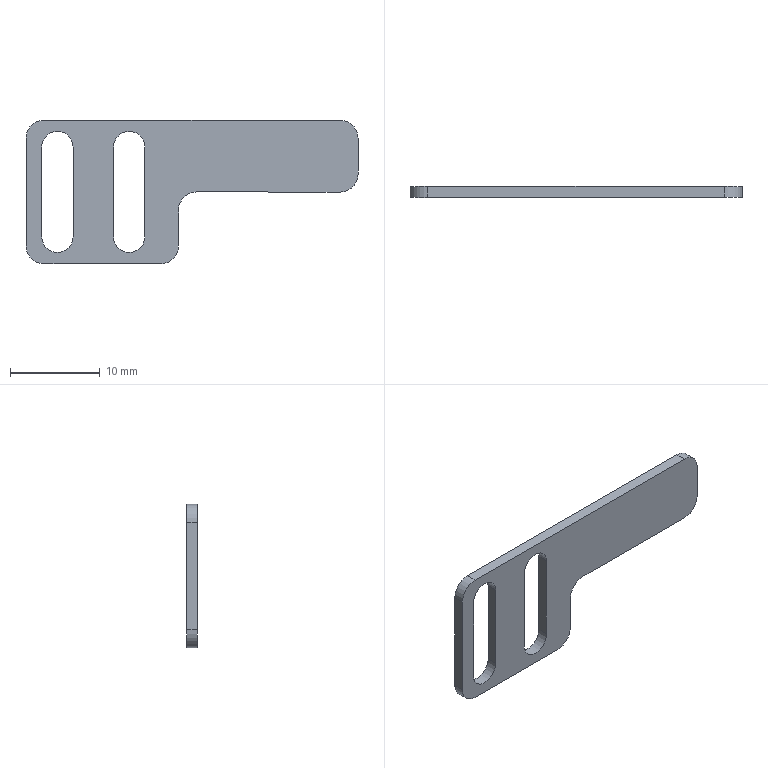Part | SolidWorks | features BaseBody 1 | 1 solid | 24 faces | box 37 x 1.2 x 16 mm | volume 407.189 mm3 | cylinder 12 | plane 12 | commonest cylinder face diameters 3.5 x6 4 x6
STEP:
#1=CARTESIAN_POINT('',(-3.5,-1.2,-8.));
#2=VERTEX_POINT('',#1);
#3=CARTESIAN_POINT('',(-1.5,-1.2,-6.));
#4=VERTEX_POINT('',#3);
#5=CARTESIAN_POINT('',(-3.5,-1.2,-6.));
#6=DIRECTION('',(0.,-1.,0.));
#7=DIRECTION('',(0.,0.,1.));
#8=AXIS2_PLACEMENT_3D('',#5,#6,#7);
#9=CIRCLE('',#8,2.);
#10=EDGE_CURVE('',#2,#4,#9,.T.);
#11=ORIENTED_EDGE('',*,*,#10,.F.);
#12=CARTESIAN_POINT('',(-3.5,0.,-8.));
#13=VERTEX_POINT('',#12);
#14=CARTESIAN_POINT('',(-3.5,-1.2,-8.));
#15=DIRECTION('',(0.,-1.,0.));
#16=VECTOR('',#15,1000.);
#17=LINE('',#14,#16);
#18=EDGE_CURVE('',#13,#2,#17,.T.);
#19=ORIENTED_EDGE('',*,*,#18,.F.);
#20=CARTESIAN_POINT('',(-1.5,0.,-6.));
#21=VERTEX_POINT('',#20);
#22=CARTESIAN_POINT('',(-3.5,0.,-6.));
#23=DIRECTION('',(0.,1.,0.));
#24=DIRECTION('',(0.,0.,1.));
#25=AXIS2_PLACEMENT_3D('',#22,#23,#24);
#26=CIRCLE('',#25,2.);
#27=EDGE_CURVE('',#21,#13,#26,.T.);
#28=ORIENTED_EDGE('',*,*,#27,.F.);
#29=CARTESIAN_POINT('',(-1.5,0.,-6.));
#30=DIRECTION('',(0.,1.,0.));
#31=VECTOR('',#30,1000.);
#32=LINE('',#29,#31);
#33=EDGE_CURVE('',#4,#21,#32,.T.);
#34=ORIENTED_EDGE('',*,*,#33,.F.);
#35=EDGE_LOOP('',(#11,#19,#28,#34));
#36=FACE_OUTER_BOUND('',#35,.T.);
#37=CARTESIAN_POINT('',(-3.5,-1.201,-6.));
#38=DIRECTION('',(0.,-1.,0.));
#39=DIRECTION('',(0.,0.,-1.));
#40=AXIS2_PLACEMENT_3D('',#37,#38,#39);
#41=CYLINDRICAL_SURFACE('',#40,2.);
#42=ADVANCED_FACE('',(#36),#41,.T.);
#43=CARTESIAN_POINT('',(16.5,-1.2,0.));
#44=VERTEX_POINT('',#43);
#45=CARTESIAN_POINT('',(18.5,-1.2,2.));
#46=VERTEX_POINT('',#45);
#47=CARTESIAN_POINT('',(16.5,-1.2,2.));
#48=DIRECTION('',(0.,-1.,0.));
#49=DIRECTION('',(0.,0.,1.));
#50=AXIS2_PLACEMENT_3D('',#47,#48,#49);
#51=CIRCLE('',#50,2.);
#52=EDGE_CURVE('',#44,#46,#51,.T.);
#53=ORIENTED_EDGE('',*,*,#52,.F.);
#54=CARTESIAN_POINT('',(16.5,0.,0.));
#55=VERTEX_POINT('',#54);
#56=CARTESIAN_POINT('',(16.5,-1.2,0.));
#57=DIRECTION('',(0.,-1.,0.));
#58=VECTOR('',#57,1000.);
#59=LINE('',#56,#58);
#60=EDGE_CURVE('',#55,#44,#59,.T.);
#61=ORIENTED_EDGE('',*,*,#60,.F.);
#62=CARTESIAN_POINT('',(18.5,0.,2.));
#63=VERTEX_POINT('',#62);
#64=CARTESIAN_POINT('',(16.5,0.,2.));
#65=DIRECTION('',(0.,1.,0.));
#66=DIRECTION('',(0.,0.,1.));
#67=AXIS2_PLACEMENT_3D('',#64,#65,#66);
#68=CIRCLE('',#67,2.);
#69=EDGE_CURVE('',#63,#55,#68,.T.);
#70=ORIENTED_EDGE('',*,*,#69,.F.);
#71=CARTESIAN_POINT('',(18.5,0.,2.));
#72=DIRECTION('',(0.,1.,0.));
#73=VECTOR('',#72,1000.);
#74=LINE('',#71,#73);
#75=EDGE_CURVE('',#46,#63,#74,.T.);
#76=ORIENTED_EDGE('',*,*,#75,.F.);
#77=EDGE_LOOP('',(#53,#61,#70,#76));
#78=FACE_OUTER_BOUND('',#77,.T.);
#79=CARTESIAN_POINT('',(16.5,-1.2,2.));
#80=DIRECTION('',(0.,-1.,0.));
#81=DIRECTION('',(0.,0.,-1.));
#82=AXIS2_PLACEMENT_3D('',#79,#80,#81);
#83=CYLINDRICAL_SURFACE('',#82,2.);
#84=ADVANCED_FACE('',(#78),#83,.T.);
#85=CARTESIAN_POINT('',(-1.5,-1.2,-2.));
#86=VERTEX_POINT('',#85);
#87=CARTESIAN_POINT('',(0.5,-1.2,0.));
#88=VERTEX_POINT('',#87);
#89=CARTESIAN_POINT('',(0.5,-1.2,-2.));
#90=DIRECTION('',(0.,1.,0.));
#91=DIRECTION('',(0.,0.,1.));
#92=AXIS2_PLACEMENT_3D('',#89,#90,#91);
#93=CIRCLE('',#92,2.);
#94=EDGE_CURVE('',#86,#88,#93,.T.);
#95=ORIENTED_EDGE('',*,*,#94,.F.);
#96=CARTESIAN_POINT('',(-1.5,0.,-2.));
#97=VERTEX_POINT('',#96);
#98=CARTESIAN_POINT('',(-1.5,-1.2,-2.));
#99=DIRECTION('',(0.,-1.,0.));
#100=VECTOR('',#99,1000.);
#101=LINE('',#98,#100);
#102=EDGE_CURVE('',#97,#86,#101,.T.);
#103=ORIENTED_EDGE('',*,*,#102,.F.);
#104=CARTESIAN_POINT('',(0.5,0.,0.));
#105=VERTEX_POINT('',#104);
#106=CARTESIAN_POINT('',(0.5,0.,-2.));
#107=DIRECTION('',(0.,-1.,0.));
#108=DIRECTION('',(0.,0.,1.));
#109=AXIS2_PLACEMENT_3D('',#106,#107,#108);
#110=CIRCLE('',#109,2.);
#111=EDGE_CURVE('',#105,#97,#110,.T.);
#112=ORIENTED_EDGE('',*,*,#111,.F.);
#113=CARTESIAN_POINT('',(0.5,0.,0.));
#114=DIRECTION('',(0.,1.,0.));
#115=VECTOR('',#114,1000.);
#116=LINE('',#113,#115);
#117=EDGE_CURVE('',#88,#105,#116,.T.);
#118=ORIENTED_EDGE('',*,*,#117,.F.);
#119=EDGE_LOOP('',(#95,#103,#112,#118));
#120=FACE_OUTER_BOUND('',#119,.T.);
#121=CARTESIAN_POINT('',(0.5,-1.201,-2.));
#122=DIRECTION('',(0.,-1.,0.));
#123=DIRECTION('',(0.,0.,-1.));
#124=AXIS2_PLACEMENT_3D('',#121,#122,#123);
#125=CYLINDRICAL_SURFACE('',#124,2.);
#126=ADVANCED_FACE('',(#120),#125,.F.);
#127=CARTESIAN_POINT('',(-18.5,-1.2,-6.));
#128=VERTEX_POINT('',#127);
#129=CARTESIAN_POINT('',(-16.5,-1.2,-8.));
#130=VERTEX_POINT('',#129);
#131=CARTESIAN_POINT('',(-16.5,-1.2,-6.));
#132=DIRECTION('',(0.,-1.,0.));
#133=DIRECTION('',(0.,0.,1.));
#134=AXIS2_PLACEMENT_3D('',#131,#132,#133);
#135=CIRCLE('',#134,2.);
#136=EDGE_CURVE('',#128,#130,#135,.T.);
#137=ORIENTED_EDGE('',*,*,#136,.F.);
#138=CARTESIAN_POINT('',(-18.5,0.,-6.));
#139=VERTEX_POINT('',#138);
#140=CARTESIAN_POINT('',(-18.5,-1.2,-6.));
#141=DIRECTION('',(0.,-1.,0.));
#142=VECTOR('',#141,1000.);
#143=LINE('',#140,#142);
#144=EDGE_CURVE('',#139,#128,#143,.T.);
#145=ORIENTED_EDGE('',*,*,#144,.F.);
#146=CARTESIAN_POINT('',(-16.5,0.,-8.));
#147=VERTEX_POINT('',#146);
#148=CARTESIAN_POINT('',(-16.5,0.,-6.));
#149=DIRECTION('',(0.,1.,0.));
#150=DIRECTION('',(0.,0.,1.));
#151=AXIS2_PLACEMENT_3D('',#148,#149,#150);
#152=CIRCLE('',#151,2.);
#153=EDGE_CURVE('',#147,#139,#152,.T.);
#154=ORIENTED_EDGE('',*,*,#153,.F.);
#155=CARTESIAN_POINT('',(-16.5,-1.2,-8.));
#156=DIRECTION('',(0.,1.,0.));
#157=VECTOR('',#156,1000.);
#158=LINE('',#155,#157);
#159=EDGE_CURVE('',#130,#147,#158,.T.);
#160=ORIENTED_EDGE('',*,*,#159,.F.);
#161=EDGE_LOOP('',(#137,#145,#154,#160));
#162=FACE_OUTER_BOUND('',#161,.T.);
#163=CARTESIAN_POINT('',(-16.5,-1.2,-6.));
#164=DIRECTION('',(0.,1.,0.));
#165=DIRECTION('',(0.,0.,1.));
#166=AXIS2_PLACEMENT_3D('',#163,#164,#165);
#167=CYLINDRICAL_SURFACE('',#166,2.);
#168=ADVANCED_FACE('',(#162),#167,.T.);
#169=CARTESIAN_POINT('',(-16.5,-1.2,8.));
#170=VERTEX_POINT('',#169);
#171=CARTESIAN_POINT('',(-18.5,-1.2,6.));
#172=VERTEX_POINT('',#171);
#173=CARTESIAN_POINT('',(-16.5,-1.2,6.));
#174=DIRECTION('',(0.,-1.,0.));
#175=DIRECTION('',(0.,0.,1.));
#176=AXIS2_PLACEMENT_3D('',#173,#174,#175);
#177=CIRCLE('',#176,2.);
#178=EDGE_CURVE('',#170,#172,#177,.T.);
#179=ORIENTED_EDGE('',*,*,#178,.F.);
#180=CARTESIAN_POINT('',(-16.5,0.,8.));
#181=VERTEX_POINT('',#180);
#182=CARTESIAN_POINT('',(-16.5,-1.2,8.));
#183=DIRECTION('',(0.,-1.,0.));
#184=VECTOR('',#183,1000.);
#185=LINE('',#182,#184);
#186=EDGE_CURVE('',#181,#170,#185,.T.);
#187=ORIENTED_EDGE('',*,*,#186,.F.);
#188=CARTESIAN_POINT('',(-18.5,0.,6.));
#189=VERTEX_POINT('',#188);
#190=CARTESIAN_POINT('',(-16.5,0.,6.));
#191=DIRECTION('',(0.,1.,0.));
#192=DIRECTION('',(0.,0.,1.));
#193=AXIS2_PLACEMENT_3D('',#190,#191,#192);
#194=CIRCLE('',#193,2.);
#195=EDGE_CURVE('',#189,#181,#194,.T.);
#196=ORIENTED_EDGE('',*,*,#195,.F.);
#197=CARTESIAN_POINT('',(-18.5,-1.2,6.));
#198=DIRECTION('',(0.,1.,0.));
#199=VECTOR('',#198,1000.);
#200=LINE('',#197,#199);
#201=EDGE_CURVE('',#172,#189,#200,.T.);
#202=ORIENTED_EDGE('',*,*,#201,.F.);
#203=EDGE_LOOP('',(#179,#187,#196,#202));
#204=FACE_OUTER_BOUND('',#203,.T.);
#205=CARTESIAN_POINT('',(-16.5,-1.2,6.));
#206=DIRECTION('',(0.,1.,0.));
#207=DIRECTION('',(0.,0.,1.));
#208=AXIS2_PLACEMENT_3D('',#205,#206,#207);
#209=CYLINDRICAL_SURFACE('',#208,2.);
#210=ADVANCED_FACE('',(#204),#209,.T.);
#211=CARTESIAN_POINT('',(18.5,-1.2,6.));
#212=VERTEX_POINT('',#211);
#213=CARTESIAN_POINT('',(16.5,-1.2,8.));
#214=VERTEX_POINT('',#213);
#215=CARTESIAN_POINT('',(16.5,-1.2,6.));
#216=DIRECTION('',(0.,-1.,0.));
#217=DIRECTION('',(0.,0.,1.));
#218=AXIS2_PLACEMENT_3D('',#215,#216,#217);
#219=CIRCLE('',#218,2.);
#220=EDGE_CURVE('',#212,#214,#219,.T.);
#221=ORIENTED_EDGE('',*,*,#220,.F.);
#222=CARTESIAN_POINT('',(18.5,0.,6.));
#223=VERTEX_POINT('',#222);
#224=CARTESIAN_POINT('',(18.5,-1.2,6.));
#225=DIRECTION('',(0.,-1.,0.));
#226=VECTOR('',#225,1000.);
#227=LINE('',#224,#226);
#228=EDGE_CURVE('',#223,#212,#227,.T.);
#229=ORIENTED_EDGE('',*,*,#228,.F.);
#230=CARTESIAN_POINT('',(16.5,0.,8.));
#231=VERTEX_POINT('',#230);
#232=CARTESIAN_POINT('',(16.5,0.,6.));
#233=DIRECTION('',(0.,1.,0.));
#234=DIRECTION('',(0.,0.,1.));
#235=AXIS2_PLACEMENT_3D('',#232,#233,#234);
#236=CIRCLE('',#235,2.);
#237=EDGE_CURVE('',#231,#223,#236,.T.);
#238=ORIENTED_EDGE('',*,*,#237,.F.);
#239=CARTESIAN_POINT('',(16.5,-1.2,8.));
#240=DIRECTION('',(0.,1.,0.));
#241=VECTOR('',#240,1000.);
#242=LINE('',#239,#241);
#243=EDGE_CURVE('',#214,#231,#242,.T.);
#244=ORIENTED_EDGE('',*,*,#243,.F.);
#245=EDGE_LOOP('',(#221,#229,#238,#244));
#246=FACE_OUTER_BOUND('',#245,.T.);
#247=CARTESIAN_POINT('',(16.5,-1.2,6.));
#248=DIRECTION('',(0.,1.,0.));
#249=DIRECTION('',(0.,0.,1.));
#250=AXIS2_PLACEMENT_3D('',#247,#248,#249);
#251=CYLINDRICAL_SURFACE('',#250,2.);
#252=ADVANCED_FACE('',(#246),#251,.T.);
#253=CARTESIAN_POINT('',(-1.5,0.,-8.));
#254=DIRECTION('',(0.,0.,1.));
#255=VECTOR('',#254,1000.);
#256=LINE('',#253,#255);
#257=EDGE_CURVE('',#21,#97,#256,.T.);
#258=ORIENTED_EDGE('',*,*,#257,.T.);
#259=ORIENTED_EDGE('',*,*,#102,.T.);
#260=CARTESIAN_POINT('',(-1.5,-1.2,-8.));
#261=DIRECTION('',(0.,0.,-1.));
#262=VECTOR('',#261,1000.);
#263=LINE('',#260,#262);
#264=EDGE_CURVE('',#86,#4,#263,.T.);
#265=ORIENTED_EDGE('',*,*,#264,.T.);
#266=ORIENTED_EDGE('',*,*,#33,.T.);
#267=EDGE_LOOP('',(#258,#259,#265,#266));
#268=FACE_OUTER_BOUND('',#267,.T.);
#269=CARTESIAN_POINT('',(-1.5,-1.201,-8.));
#270=DIRECTION('',(-1.,0.,0.));
#271=DIRECTION('',(0.,1.,0.));
#272=AXIS2_PLACEMENT_3D('',#269,#270,#271);
#273=PLANE('',#272);
#274=ADVANCED_FACE('',(#268),#273,.F.);
#275=CARTESIAN_POINT('',(18.5,-1.2,0.));
#276=DIRECTION('',(-1.,0.,0.));
#277=VECTOR('',#276,1000.);
#278=LINE('',#275,#277);
#279=EDGE_CURVE('',#44,#88,#278,.T.);
#280=ORIENTED_EDGE('',*,*,#279,.T.);
#281=ORIENTED_EDGE('',*,*,#117,.T.);
#282=CARTESIAN_POINT('',(18.5,0.,0.));
#283=DIRECTION('',(1.,0.,0.));
#284=VECTOR('',#283,1000.);
#285=LINE('',#282,#284);
#286=EDGE_CURVE('',#105,#55,#285,.T.);
#287=ORIENTED_EDGE('',*,*,#286,.T.);
#288=ORIENTED_EDGE('',*,*,#60,.T.);
#289=EDGE_LOOP('',(#280,#281,#287,#288));
#290=FACE_OUTER_BOUND('',#289,.T.);
#291=CARTESIAN_POINT('',(18.5,-1.201,0.));
#292=DIRECTION('',(0.,0.,1.));
#293=DIRECTION('',(1.,0.,0.));
#294=AXIS2_PLACEMENT_3D('',#291,#292,#293);
#295=PLANE('',#294);
#296=ADVANCED_FACE('',(#290),#295,.F.);
#297=CARTESIAN_POINT('',(-16.75,-1.2,5.));
#298=VERTEX_POINT('',#297);
#299=CARTESIAN_POINT('',(-16.75,-1.2,-5.));
#300=VERTEX_POINT('',#299);
#301=CARTESIAN_POINT('',(-16.75,-1.2,-5.));
#302=DIRECTION('',(0.,0.,-1.));
#303=VECTOR('',#302,1000.);
#304=LINE('',#301,#303);
#305=EDGE_CURVE('',#298,#300,#304,.T.);
#306=ORIENTED_EDGE('',*,*,#305,.T.);
#307=CARTESIAN_POINT('',(-16.75,0.,-5.));
#308=VERTEX_POINT('',#307);
#309=CARTESIAN_POINT('',(-16.75,-1.201,-5.));
#310=DIRECTION('',(0.,1.,0.));
#311=VECTOR('',#310,1000.);
#312=LINE('',#309,#311);
#313=EDGE_CURVE('',#300,#308,#312,.T.);
#314=ORIENTED_EDGE('',*,*,#313,.T.);
#315=CARTESIAN_POINT('',(-16.75,0.,5.));
#316=VERTEX_POINT('',#315);
#317=CARTESIAN_POINT('',(-16.75,0.,-5.));
#318=DIRECTION('',(0.,0.,1.));
#319=VECTOR('',#318,1000.);
#320=LINE('',#317,#319);
#321=EDGE_CURVE('',#308,#316,#320,.T.);
#322=ORIENTED_EDGE('',*,*,#321,.T.);
#323=CARTESIAN_POINT('',(-16.75,-1.201,5.));
#324=DIRECTION('',(0.,1.,0.));
#325=VECTOR('',#324,1000.);
#326=LINE('',#323,#325);
#327=EDGE_CURVE('',#298,#316,#326,.T.);
#328=ORIENTED_EDGE('',*,*,#327,.F.);
#329=EDGE_LOOP('',(#306,#314,#322,#328));
#330=FACE_OUTER_BOUND('',#329,.T.);
#331=CARTESIAN_POINT('',(-16.75,-1.201,-5.));
#332=DIRECTION('',(-1.,0.,0.));
#333=DIRECTION('',(0.,0.,1.));
#334=AXIS2_PLACEMENT_3D('',#331,#332,#333);
#335=PLANE('',#334);
#336=ADVANCED_FACE('',(#330),#335,.F.);
#337=CARTESIAN_POINT('',(-15.,-1.2,6.75));
#338=VERTEX_POINT('',#337);
#339=CARTESIAN_POINT('',(-15.,0.,6.75));
#340=VERTEX_POINT('',#339);
#341=CARTESIAN_POINT('',(-15.,-1.201,6.75));
#342=DIRECTION('',(0.,1.,0.));
#343=VECTOR('',#342,1000.);
#344=LINE('',#341,#343);
#345=EDGE_CURVE('',#338,#340,#344,.T.);
#346=ORIENTED_EDGE('',*,*,#345,.F.);
#347=CARTESIAN_POINT('',(-15.,-1.2,5.));
#348=DIRECTION('',(0.,-1.,0.));
#349=DIRECTION('',(0.,0.,1.));
#350=AXIS2_PLACEMENT_3D('',#347,#348,#349);
#351=CIRCLE('',#350,1.75);
#352=EDGE_CURVE('',#338,#298,#351,.T.);
#353=ORIENTED_EDGE('',*,*,#352,.T.);
#354=ORIENTED_EDGE('',*,*,#327,.T.);
#355=CARTESIAN_POINT('',(-15.,0.,5.));
#356=DIRECTION('',(0.,1.,0.));
#357=DIRECTION('',(0.,0.,1.));
#358=AXIS2_PLACEMENT_3D('',#355,#356,#357);
#359=CIRCLE('',#358,1.75);
#360=EDGE_CURVE('',#316,#340,#359,.T.);
#361=ORIENTED_EDGE('',*,*,#360,.T.);
#362=EDGE_LOOP('',(#346,#353,#354,#361));
#363=FACE_OUTER_BOUND('',#362,.T.);
#364=CARTESIAN_POINT('',(-15.,-1.201,5.));
#365=DIRECTION('',(0.,1.,0.));
#366=DIRECTION('',(0.,0.,1.));
#367=AXIS2_PLACEMENT_3D('',#364,#365,#366);
#368=CYLINDRICAL_SURFACE('',#367,1.75);
#369=ADVANCED_FACE('',(#363),#368,.F.);
#370=CARTESIAN_POINT('',(-13.25,-1.2,-5.));
#371=VERTEX_POINT('',#370);
#372=CARTESIAN_POINT('',(-13.25,-1.2,5.));
#373=VERTEX_POINT('',#372);
#374=CARTESIAN_POINT('',(-13.25,-1.2,-5.));
#375=DIRECTION('',(0.,0.,1.));
#376=VECTOR('',#375,1000.);
#377=LINE('',#374,#376);
#378=EDGE_CURVE('',#371,#373,#377,.T.);
#379=ORIENTED_EDGE('',*,*,#378,.T.);
#380=CARTESIAN_POINT('',(-13.25,0.,5.));
#381=VERTEX_POINT('',#380);
#382=CARTESIAN_POINT('',(-13.25,-1.201,5.));
#383=DIRECTION('',(0.,1.,0.));
#384=VECTOR('',#383,1000.);
#385=LINE('',#382,#384);
#386=EDGE_CURVE('',#373,#381,#385,.T.);
#387=ORIENTED_EDGE('',*,*,#386,.T.);
#388=CARTESIAN_POINT('',(-13.25,0.,-5.));
#389=VERTEX_POINT('',#388);
#390=CARTESIAN_POINT('',(-13.25,0.,-5.));
#391=DIRECTION('',(0.,0.,-1.));
#392=VECTOR('',#391,1000.);
#393=LINE('',#390,#392);
#394=EDGE_CURVE('',#381,#389,#393,.T.);
#395=ORIENTED_EDGE('',*,*,#394,.T.);
#396=CARTESIAN_POINT('',(-13.25,-1.201,-5.));
#397=DIRECTION('',(0.,1.,0.));
#398=VECTOR('',#397,1000.);
#399=LINE('',#396,#398);
#400=EDGE_CURVE('',#371,#389,#399,.T.);
#401=ORIENTED_EDGE('',*,*,#400,.F.);
#402=EDGE_LOOP('',(#379,#387,#395,#401));
#403=FACE_OUTER_BOUND('',#402,.T.);
#404=CARTESIAN_POINT('',(-13.25,-1.201,-5.));
#405=DIRECTION('',(1.,0.,0.));
#406=DIRECTION('',(0.,1.,0.));
#407=AXIS2_PLACEMENT_3D('',#404,#405,#406);
#408=PLANE('',#407);
#409=ADVANCED_FACE('',(#403),#408,.F.);
#410=CARTESIAN_POINT('',(-15.,-1.2,-5.));
#411=DIRECTION('',(0.,-1.,0.));
#412=DIRECTION('',(0.,0.,1.));
#413=AXIS2_PLACEMENT_3D('',#410,#411,#412);
#414=CIRCLE('',#413,1.75);
#415=EDGE_CURVE('',#300,#371,#414,.T.);
#416=ORIENTED_EDGE('',*,*,#415,.T.);
#417=ORIENTED_EDGE('',*,*,#400,.T.);
#418=CARTESIAN_POINT('',(-15.,0.,-5.));
#419=DIRECTION('',(0.,1.,0.));
#420=DIRECTION('',(0.,0.,1.));
#421=AXIS2_PLACEMENT_3D('',#418,#419,#420);
#422=CIRCLE('',#421,1.75);
#423=EDGE_CURVE('',#389,#308,#422,.T.);
#424=ORIENTED_EDGE('',*,*,#423,.T.);
#425=ORIENTED_EDGE('',*,*,#313,.F.);
#426=EDGE_LOOP('',(#416,#417,#424,#425));
#427=FACE_OUTER_BOUND('',#426,.T.);
#428=CARTESIAN_POINT('',(-15.,-1.201,-5.));
#429=DIRECTION('',(0.,1.,0.));
#430=DIRECTION('',(0.,0.,1.));
#431=AXIS2_PLACEMENT_3D('',#428,#429,#430);
#432=CYLINDRICAL_SURFACE('',#431,1.75);
#433=ADVANCED_FACE('',(#427),#432,.F.);
#434=CARTESIAN_POINT('',(-8.75,-1.2,5.));
#435=VERTEX_POINT('',#434);
#436=CARTESIAN_POINT('',(-8.75,-1.2,-5.));
#437=VERTEX_POINT('',#436);
#438=CARTESIAN_POINT('',(-8.75,-1.2,-5.));
#439=DIRECTION('',(0.,0.,-1.));
#440=VECTOR('',#439,1000.);
#441=LINE('',#438,#440);
#442=EDGE_CURVE('',#435,#437,#441,.T.);
#443=ORIENTED_EDGE('',*,*,#442,.T.);
#444=CARTESIAN_POINT('',(-8.75,0.,-5.));
#445=VERTEX_POINT('',#444);
#446=CARTESIAN_POINT('',(-8.75,-1.201,-5.));
#447=DIRECTION('',(0.,1.,0.));
#448=VECTOR('',#447,1000.);
#449=LINE('',#446,#448);
#450=EDGE_CURVE('',#437,#445,#449,.T.);
#451=ORIENTED_EDGE('',*,*,#450,.T.);
#452=CARTESIAN_POINT('',(-8.75,0.,5.));
#453=VERTEX_POINT('',#452);
#454=CARTESIAN_POINT('',(-8.75,0.,-5.));
#455=DIRECTION('',(0.,0.,1.));
#456=VECTOR('',#455,1000.);
#457=LINE('',#454,#456);
#458=EDGE_CURVE('',#445,#453,#457,.T.);
#459=ORIENTED_EDGE('',*,*,#458,.T.);
#460=CARTESIAN_POINT('',(-8.75,-1.201,5.));
#461=DIRECTION('',(0.,1.,0.));
#462=VECTOR('',#461,1000.);
#463=LINE('',#460,#462);
#464=EDGE_CURVE('',#435,#453,#463,.T.);
#465=ORIENTED_EDGE('',*,*,#464,.F.);
#466=EDGE_LOOP('',(#443,#451,#459,#465));
#467=FACE_OUTER_BOUND('',#466,.T.);
#468=CARTESIAN_POINT('',(-8.75,-1.201,-5.));
#469=DIRECTION('',(-1.,0.,0.));
#470=DIRECTION('',(0.,0.,1.));
#471=AXIS2_PLACEMENT_3D('',#468,#469,#470);
#472=PLANE('',#471);
#473=ADVANCED_FACE('',(#467),#472,.F.);
#474=CARTESIAN_POINT('',(-7.,-1.2,6.75));
#475=VERTEX_POINT('',#474);
#476=CARTESIAN_POINT('',(-7.,0.,6.75));
#477=VERTEX_POINT('',#476);
#478=CARTESIAN_POINT('',(-7.,-1.201,6.75));
#479=DIRECTION('',(0.,1.,0.));
#480=VECTOR('',#479,1000.);
#481=LINE('',#478,#480);
#482=EDGE_CURVE('',#475,#477,#481,.T.);
#483=ORIENTED_EDGE('',*,*,#482,.F.);
#484=CARTESIAN_POINT('',(-7.,-1.2,5.));
#485=DIRECTION('',(0.,-1.,0.));
#486=DIRECTION('',(0.,0.,1.));
#487=AXIS2_PLACEMENT_3D('',#484,#485,#486);
#488=CIRCLE('',#487,1.75);
#489=EDGE_CURVE('',#475,#435,#488,.T.);
#490=ORIENTED_EDGE('',*,*,#489,.T.);
#491=ORIENTED_EDGE('',*,*,#464,.T.);
#492=CARTESIAN_POINT('',(-7.,0.,5.));
#493=DIRECTION('',(0.,1.,0.));
#494=DIRECTION('',(0.,0.,1.));
#495=AXIS2_PLACEMENT_3D('',#492,#493,#494);
#496=CIRCLE('',#495,1.75);
#497=EDGE_CURVE('',#453,#477,#496,.T.);
#498=ORIENTED_EDGE('',*,*,#497,.T.);
#499=EDGE_LOOP('',(#483,#490,#491,#498));
#500=FACE_OUTER_BOUND('',#499,.T.);
#501=CARTESIAN_POINT('',(-7.,-1.201,5.));
#502=DIRECTION('',(0.,1.,0.));
#503=DIRECTION('',(0.,0.,1.));
#504=AXIS2_PLACEMENT_3D('',#501,#502,#503);
#505=CYLINDRICAL_SURFACE('',#504,1.75);
#506=ADVANCED_FACE('',(#500),#505,.F.);
#507=CARTESIAN_POINT('',(-5.25,-1.2,-5.));
#508=VERTEX_POINT('',#507);
#509=CARTESIAN_POINT('',(-5.25,-1.2,5.));
#510=VERTEX_POINT('',#509);
#511=CARTESIAN_POINT('',(-5.25,-1.2,-5.));
#512=DIRECTION('',(0.,0.,1.));
#513=VECTOR('',#512,1000.);
#514=LINE('',#511,#513);
#515=EDGE_CURVE('',#508,#510,#514,.T.);
#516=ORIENTED_EDGE('',*,*,#515,.T.);
#517=CARTESIAN_POINT('',(-5.25,0.,5.));
#518=VERTEX_POINT('',#517);
#519=CARTESIAN_POINT('',(-5.25,-1.201,5.));
#520=DIRECTION('',(0.,1.,0.));
#521=VECTOR('',#520,1000.);
#522=LINE('',#519,#521);
#523=EDGE_CURVE('',#510,#518,#522,.T.);
#524=ORIENTED_EDGE('',*,*,#523,.T.);
#525=CARTESIAN_POINT('',(-5.25,0.,-5.));
#526=VERTEX_POINT('',#525);
#527=CARTESIAN_POINT('',(-5.25,0.,-5.));
#528=DIRECTION('',(0.,0.,-1.));
#529=VECTOR('',#528,1000.);
#530=LINE('',#527,#529);
#531=EDGE_CURVE('',#518,#526,#530,.T.);
#532=ORIENTED_EDGE('',*,*,#531,.T.);
#533=CARTESIAN_POINT('',(-5.25,-1.201,-5.));
#534=DIRECTION('',(0.,1.,0.));
#535=VECTOR('',#534,1000.);
#536=LINE('',#533,#535);
#537=EDGE_CURVE('',#508,#526,#536,.T.);
#538=ORIENTED_EDGE('',*,*,#537,.F.);
#539=EDGE_LOOP('',(#516,#524,#532,#538));
#540=FACE_OUTER_BOUND('',#539,.T.);
#541=CARTESIAN_POINT('',(-5.25,-1.201,-5.));
#542=DIRECTION('',(1.,0.,0.));
#543=DIRECTION('',(0.,1.,0.));
#544=AXIS2_PLACEMENT_3D('',#541,#542,#543);
#545=PLANE('',#544);
#546=ADVANCED_FACE('',(#540),#545,.F.);
#547=CARTESIAN_POINT('',(-7.,-1.2,-5.));
#548=DIRECTION('',(0.,-1.,0.));
#549=DIRECTION('',(0.,0.,1.));
#550=AXIS2_PLACEMENT_3D('',#547,#548,#549);
#551=CIRCLE('',#550,1.75);
#552=EDGE_CURVE('',#437,#508,#551,.T.);
#553=ORIENTED_EDGE('',*,*,#552,.T.);
#554=ORIENTED_EDGE('',*,*,#537,.T.);
#555=CARTESIAN_POINT('',(-7.,0.,-5.));
#556=DIRECTION('',(0.,1.,0.));
#557=DIRECTION('',(0.,0.,1.));
#558=AXIS2_PLACEMENT_3D('',#555,#556,#557);
#559=CIRCLE('',#558,1.75);
#560=EDGE_CURVE('',#526,#445,#559,.T.);
#561=ORIENTED_EDGE('',*,*,#560,.T.);
#562=ORIENTED_EDGE('',*,*,#450,.F.);
#563=EDGE_LOOP('',(#553,#554,#561,#562));
#564=FACE_OUTER_BOUND('',#563,.T.);
#565=CARTESIAN_POINT('',(-7.,-1.201,-5.));
#566=DIRECTION('',(0.,1.,0.));
#567=DIRECTION('',(0.,0.,1.));
#568=AXIS2_PLACEMENT_3D('',#565,#566,#567);
#569=CYLINDRICAL_SURFACE('',#568,1.75);
#570=ADVANCED_FACE('',(#564),#569,.F.);
#571=ORIENTED_EDGE('',*,*,#560,.F.);
#572=ORIENTED_EDGE('',*,*,#531,.F.);
#573=CARTESIAN_POINT('',(-7.,0.,5.));
#574=DIRECTION('',(0.,1.,0.));
#575=DIRECTION('',(0.,0.,1.));
#576=AXIS2_PLACEMENT_3D('',#573,#574,#575);
#577=CIRCLE('',#576,1.75);
#578=EDGE_CURVE('',#477,#518,#577,.T.);
#579=ORIENTED_EDGE('',*,*,#578,.F.);
#580=ORIENTED_EDGE('',*,*,#497,.F.);
#581=ORIENTED_EDGE('',*,*,#458,.F.);
#582=EDGE_LOOP('',(#571,#572,#579,#580,#581));
#583=FACE_BOUND('',#582,.T.);
#584=ORIENTED_EDGE('',*,*,#423,.F.);
#585=ORIENTED_EDGE('',*,*,#394,.F.);
#586=CARTESIAN_POINT('',(-15.,0.,5.));
#587=DIRECTION('',(0.,1.,0.));
#588=DIRECTION('',(0.,0.,1.));
#589=AXIS2_PLACEMENT_3D('',#586,#587,#588);
#590=CIRCLE('',#589,1.75);
#591=EDGE_CURVE('',#340,#381,#590,.T.);
#592=ORIENTED_EDGE('',*,*,#591,.F.);
#593=ORIENTED_EDGE('',*,*,#360,.F.);
#594=ORIENTED_EDGE('',*,*,#321,.F.);
#595=EDGE_LOOP('',(#584,#585,#592,#593,#594));
#596=FACE_BOUND('',#595,.T.);
#597=CARTESIAN_POINT('',(-18.5,0.,8.));
#598=DIRECTION('',(1.,0.,0.));
#599=VECTOR('',#598,1000.);
#600=LINE('',#597,#599);
#601=EDGE_CURVE('',#181,#231,#600,.T.);
#602=ORIENTED_EDGE('',*,*,#601,.T.);
#603=ORIENTED_EDGE('',*,*,#237,.T.);
#604=CARTESIAN_POINT('',(18.5,0.,-8.));
#605=DIRECTION('',(0.,0.,-1.));
#606=VECTOR('',#605,1000.);
#607=LINE('',#604,#606);
#608=EDGE_CURVE('',#223,#63,#607,.T.);
#609=ORIENTED_EDGE('',*,*,#608,.T.);
#610=ORIENTED_EDGE('',*,*,#69,.T.);
#611=ORIENTED_EDGE('',*,*,#286,.F.);
#612=ORIENTED_EDGE('',*,*,#111,.T.);
#613=ORIENTED_EDGE('',*,*,#257,.F.);
#614=ORIENTED_EDGE('',*,*,#27,.T.);
#615=CARTESIAN_POINT('',(-18.5,0.,-8.));
#616=DIRECTION('',(-1.,0.,0.));
#617=VECTOR('',#616,1000.);
#618=LINE('',#615,#617);
#619=EDGE_CURVE('',#13,#147,#618,.T.);
#620=ORIENTED_EDGE('',*,*,#619,.T.);
#621=ORIENTED_EDGE('',*,*,#153,.T.);
#622=CARTESIAN_POINT('',(-18.5,0.,-8.));
#623=DIRECTION('',(0.,0.,1.));
#624=VECTOR('',#623,1000.);
#625=LINE('',#622,#624);
#626=EDGE_CURVE('',#139,#189,#625,.T.);
#627=ORIENTED_EDGE('',*,*,#626,.T.);
#628=ORIENTED_EDGE('',*,*,#195,.T.);
#629=EDGE_LOOP('',(#602,#603,#609,#610,#611,#612,#613,#614,#620,#621,#627,#628));
#630=FACE_OUTER_BOUND('',#629,.T.);
#631=CARTESIAN_POINT('',(0.,0.,0.));
#632=DIRECTION('',(0.,1.,0.));
#633=DIRECTION('',(1.,0.,0.));
#634=AXIS2_PLACEMENT_3D('',#631,#632,#633);
#635=PLANE('',#634);
#636=ADVANCED_FACE('',(#583,#596,#630),#635,.T.);
#637=ORIENTED_EDGE('',*,*,#515,.F.);
#638=ORIENTED_EDGE('',*,*,#552,.F.);
#639=ORIENTED_EDGE('',*,*,#442,.F.);
#640=ORIENTED_EDGE('',*,*,#489,.F.);
#641=CARTESIAN_POINT('',(-7.,-1.2,5.));
#642=DIRECTION('',(0.,-1.,0.));
#643=DIRECTION('',(0.,0.,1.));
#644=AXIS2_PLACEMENT_3D('',#641,#642,#643);
#645=CIRCLE('',#644,1.75);
#646=EDGE_CURVE('',#510,#475,#645,.T.);
#647=ORIENTED_EDGE('',*,*,#646,.F.);
#648=EDGE_LOOP('',(#637,#638,#639,#640,#647));
#649=FACE_BOUND('',#648,.T.);
#650=ORIENTED_EDGE('',*,*,#378,.F.);
#651=ORIENTED_EDGE('',*,*,#415,.F.);
#652=ORIENTED_EDGE('',*,*,#305,.F.);
#653=ORIENTED_EDGE('',*,*,#352,.F.);
#654=CARTESIAN_POINT('',(-15.,-1.2,5.));
#655=DIRECTION('',(0.,-1.,0.));
#656=DIRECTION('',(0.,0.,1.));
#657=AXIS2_PLACEMENT_3D('',#654,#655,#656);
#658=CIRCLE('',#657,1.75);
#659=EDGE_CURVE('',#373,#338,#658,.T.);
#660=ORIENTED_EDGE('',*,*,#659,.F.);
#661=EDGE_LOOP('',(#650,#651,#652,#653,#660));
#662=FACE_BOUND('',#661,.T.);
#663=CARTESIAN_POINT('',(18.5,-1.2,-8.));
#664=DIRECTION('',(0.,0.,-1.));
#665=VECTOR('',#664,1000.);
#666=LINE('',#663,#665);
#667=EDGE_CURVE('',#212,#46,#666,.T.);
#668=ORIENTED_EDGE('',*,*,#667,.F.);
#669=ORIENTED_EDGE('',*,*,#220,.T.);
#670=CARTESIAN_POINT('',(-18.5,-1.2,8.));
#671=DIRECTION('',(1.,0.,0.));
#672=VECTOR('',#671,1000.);
#673=LINE('',#670,#672);
#674=EDGE_CURVE('',#170,#214,#673,.T.);
#675=ORIENTED_EDGE('',*,*,#674,.F.);
#676=ORIENTED_EDGE('',*,*,#178,.T.);
#677=CARTESIAN_POINT('',(-18.5,-1.2,-8.));
#678=DIRECTION('',(0.,0.,1.));
#679=VECTOR('',#678,1000.);
#680=LINE('',#677,#679);
#681=EDGE_CURVE('',#128,#172,#680,.T.);
#682=ORIENTED_EDGE('',*,*,#681,.F.);
#683=ORIENTED_EDGE('',*,*,#136,.T.);
#684=CARTESIAN_POINT('',(-18.5,-1.2,-8.));
#685=DIRECTION('',(-1.,0.,0.));
#686=VECTOR('',#685,1000.);
#687=LINE('',#684,#686);
#688=EDGE_CURVE('',#2,#130,#687,.T.);
#689=ORIENTED_EDGE('',*,*,#688,.F.);
#690=ORIENTED_EDGE('',*,*,#10,.T.);
#691=ORIENTED_EDGE('',*,*,#264,.F.);
#692=ORIENTED_EDGE('',*,*,#94,.T.);
#693=ORIENTED_EDGE('',*,*,#279,.F.);
#694=ORIENTED_EDGE('',*,*,#52,.T.);
#695=EDGE_LOOP('',(#668,#669,#675,#676,#682,#683,#689,#690,#691,#692,#693,#694));
#696=FACE_OUTER_BOUND('',#695,.T.);
#697=CARTESIAN_POINT('',(0.,-1.2,0.));
#698=DIRECTION('',(0.,1.,0.));
#699=DIRECTION('',(1.,0.,0.));
#700=AXIS2_PLACEMENT_3D('',#697,#698,#699);
#701=PLANE('',#700);
#702=ADVANCED_FACE('',(#649,#662,#696),#701,.F.);
#703=ORIENTED_EDGE('',*,*,#688,.T.);
#704=ORIENTED_EDGE('',*,*,#159,.T.);
#705=ORIENTED_EDGE('',*,*,#619,.F.);
#706=ORIENTED_EDGE('',*,*,#18,.T.);
#707=EDGE_LOOP('',(#703,#704,#705,#706));
#708=FACE_OUTER_BOUND('',#707,.T.);
#709=CARTESIAN_POINT('',(-18.5,-1.2,-8.));
#710=DIRECTION('',(0.,0.,-1.));
#711=DIRECTION('',(0.,-1.,0.));
#712=AXIS2_PLACEMENT_3D('',#709,#710,#711);
#713=PLANE('',#712);
#714=ADVANCED_FACE('',(#708),#713,.T.);
#715=ORIENTED_EDGE('',*,*,#681,.T.);
#716=ORIENTED_EDGE('',*,*,#201,.T.);
#717=ORIENTED_EDGE('',*,*,#626,.F.);
#718=ORIENTED_EDGE('',*,*,#144,.T.);
#719=EDGE_LOOP('',(#715,#716,#717,#718));
#720=FACE_OUTER_BOUND('',#719,.T.);
#721=CARTESIAN_POINT('',(-18.5,-1.2,-8.));
#722=DIRECTION('',(-1.,0.,0.));
#723=DIRECTION('',(0.,1.,0.));
#724=AXIS2_PLACEMENT_3D('',#721,#722,#723);
#725=PLANE('',#724);
#726=ADVANCED_FACE('',(#720),#725,.T.);
#727=ORIENTED_EDGE('',*,*,#674,.T.);
#728=ORIENTED_EDGE('',*,*,#243,.T.);
#729=ORIENTED_EDGE('',*,*,#601,.F.);
#730=ORIENTED_EDGE('',*,*,#186,.T.);
#731=EDGE_LOOP('',(#727,#728,#729,#730));
#732=FACE_OUTER_BOUND('',#731,.T.);
#733=CARTESIAN_POINT('',(-18.5,-1.2,8.));
#734=DIRECTION('',(0.,0.,1.));
#735=DIRECTION('',(1.,0.,0.));
#736=AXIS2_PLACEMENT_3D('',#733,#734,#735);
#737=PLANE('',#736);
#738=ADVANCED_FACE('',(#732),#737,.T.);
#739=ORIENTED_EDGE('',*,*,#608,.F.);
#740=ORIENTED_EDGE('',*,*,#228,.T.);
#741=ORIENTED_EDGE('',*,*,#667,.T.);
#742=ORIENTED_EDGE('',*,*,#75,.T.);
#743=EDGE_LOOP('',(#739,#740,#741,#742));
#744=FACE_OUTER_BOUND('',#743,.T.);
#745=CARTESIAN_POINT('',(18.5,-1.2,-8.));
#746=DIRECTION('',(1.,0.,0.));
#747=DIRECTION('',(0.,0.,1.));
#748=AXIS2_PLACEMENT_3D('',#745,#746,#747);
#749=PLANE('',#748);
#750=ADVANCED_FACE('',(#744),#749,.T.);
#751=ORIENTED_EDGE('',*,*,#646,.T.);
#752=ORIENTED_EDGE('',*,*,#482,.T.);
#753=ORIENTED_EDGE('',*,*,#578,.T.);
#754=ORIENTED_EDGE('',*,*,#523,.F.);
#755=EDGE_LOOP('',(#751,#752,#753,#754));
#756=FACE_OUTER_BOUND('',#755,.T.);
#757=CARTESIAN_POINT('',(-7.,-1.201,5.));
#758=DIRECTION('',(0.,1.,0.));
#759=DIRECTION('',(0.,0.,1.));
#760=AXIS2_PLACEMENT_3D('',#757,#758,#759);
#761=CYLINDRICAL_SURFACE('',#760,1.75);
#762=ADVANCED_FACE('',(#756),#761,.F.);
#763=ORIENTED_EDGE('',*,*,#659,.T.);
#764=ORIENTED_EDGE('',*,*,#345,.T.);
#765=ORIENTED_EDGE('',*,*,#591,.T.);
#766=ORIENTED_EDGE('',*,*,#386,.F.);
#767=EDGE_LOOP('',(#763,#764,#765,#766));
#768=FACE_OUTER_BOUND('',#767,.T.);
#769=CARTESIAN_POINT('',(-15.,-1.201,5.));
#770=DIRECTION('',(0.,1.,0.));
#771=DIRECTION('',(0.,0.,1.));
#772=AXIS2_PLACEMENT_3D('',#769,#770,#771);
#773=CYLINDRICAL_SURFACE('',#772,1.75);
#774=ADVANCED_FACE('',(#768),#773,.F.);
#775=CLOSED_SHELL('',(#42,#84,#126,#168,#210,#252,#274,#296,#336,#369,#409,#433,#473,#506,#546,#570,#636,#702,#714,#726,#738,#750,#762,#774));
#776=MANIFOLD_SOLID_BREP('',#775);
#777=CARTESIAN_POINT('',(0.,0.,0.));
#778=DIRECTION('',(0.,0.,1.));
#779=DIRECTION('',(1.,0.,0.));
#780=AXIS2_PLACEMENT_3D('',#777,#778,#779);
#781=(LENGTH_UNIT()NAMED_UNIT(*)SI_UNIT(.MILLI.,.METRE.));
#782=UNCERTAINTY_MEASURE_WITH_UNIT(LENGTH_MEASURE(0.00001),#781,'','');
#783=(NAMED_UNIT(*)PLANE_ANGLE_UNIT()SI_UNIT($,.RADIAN.));
#784=(NAMED_UNIT(*)SI_UNIT($,.STERADIAN.)SOLID_ANGLE_UNIT());
#785=(GEOMETRIC_REPRESENTATION_CONTEXT(3)GLOBAL_UNCERTAINTY_ASSIGNED_CONTEXT((#782))GLOBAL_UNIT_ASSIGNED_CONTEXT((#781,#783,#784))REPRESENTATION_CONTEXT('',''));
#786=ADVANCED_BREP_SHAPE_REPRESENTATION('',(#776,#780),#785);